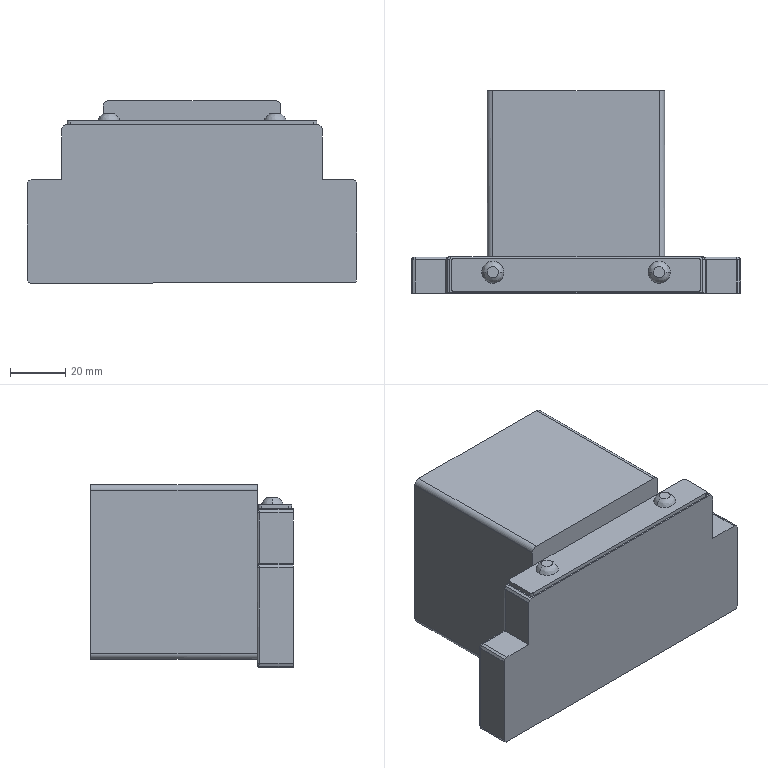Part | SolidWorks | features BaseBody 1 | 1 solid | 79 faces | box 118.964 x 73 x 66 mm | volume 247218 mm3 | plane 44 | cylinder 31 | spline 4 | commonest cylinder face diameters 2 x23 4 x4 40 x2 50.2 x2